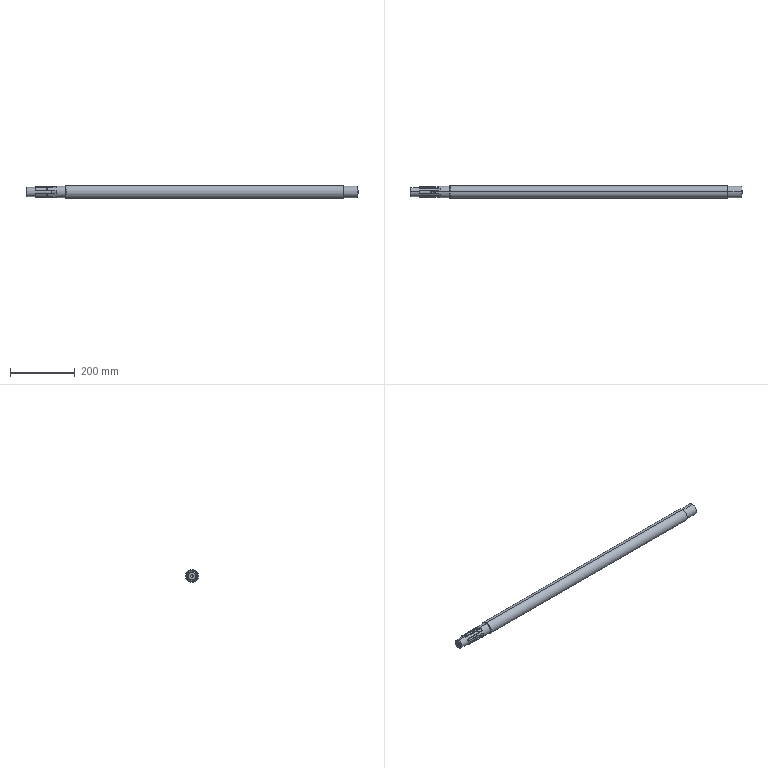Part | SolidWorks | features BaseBody 1 | 1 solid | 180 faces | box 1025 x 40 x 40 mm | volume 1210935 mm3 | cone 62 | plane 49 | cylinder 35 | spline 34 | commonest cylinder face diameters 0.2 x14 34 x7 8.376 x4 35 x4 8 x2 28 x2